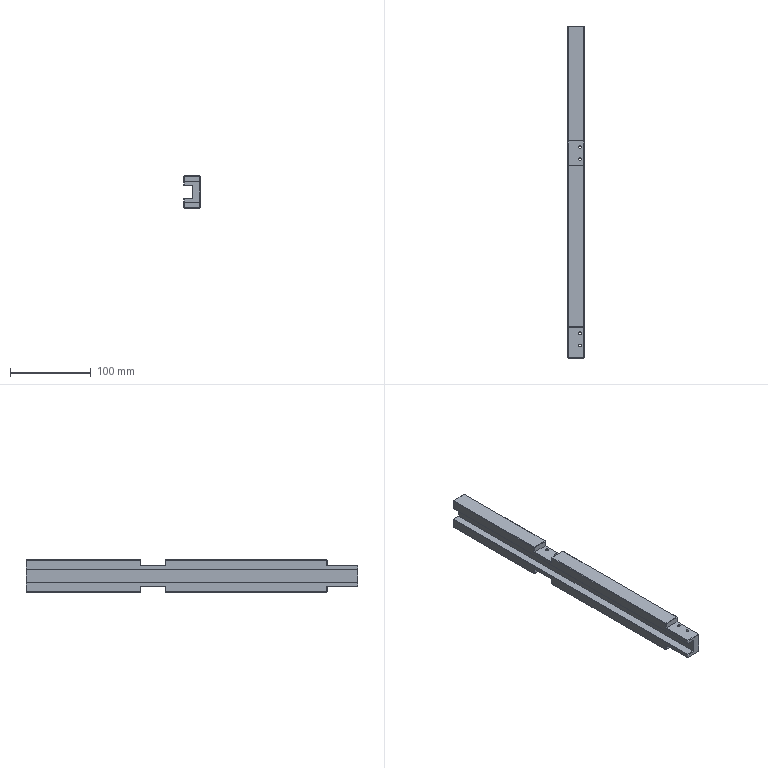Part | SolidWorks | features ICE 3, Chamfer 1, Extrusion 1, HoleWzd 1 | 1 solid | 106 faces | box 20 x 410 x 40 mm | volume 242107 mm3 | plane 98 | cylinder 8 | commonest cylinder face diameters 3.3 x8